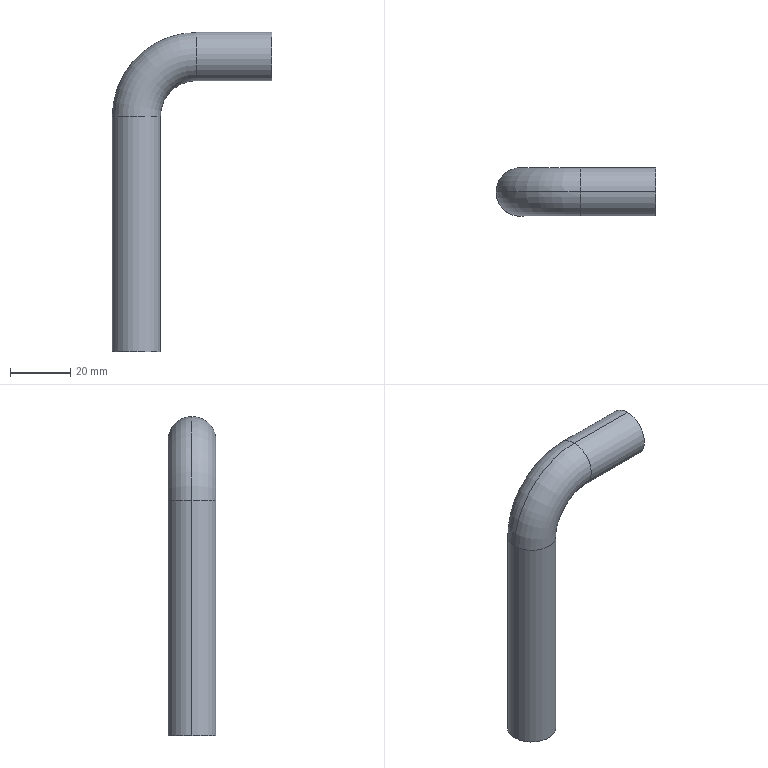Part | STEP file | copper tube 44 | 1 solid | 14 faces | box 53 x 16 x 106 mm | volume 7500 mm3 | cylinder 8 | torus 4 | plane 2 | commonest cylinder face diameters 13.6 x4 16 x4
STEP:
#1=CARTESIAN_POINT('',(0.,0.,0.));
#2=DIRECTION('',(0.,0.,1.));
#3=DIRECTION('',(1.,0.,0.));
#4=AXIS2_PLACEMENT_3D('',#1,#2,#3);
#5=CARTESIAN_POINT('',(6.8,0.,78.));
#6=VERTEX_POINT('',#5);
#7=CARTESIAN_POINT('',(20.,0.,91.2));
#8=VERTEX_POINT('',#7);
#9=CARTESIAN_POINT('',(20.,0.,78.));
#10=DIRECTION('',(0.,1.,0.));
#11=DIRECTION('',(0.,0.,1.));
#12=AXIS2_PLACEMENT_3D('',#9,#10,#11);
#13=CIRCLE('',#12,13.2);
#14=CARTESIAN_POINT('',(20.,0.,78.));
#15=DIRECTION('',(0.,1.,0.));
#16=DIRECTION('',(0.,0.,1.));
#17=AXIS2_PLACEMENT_3D('',#14,#15,#16);
#18=TOROIDAL_SURFACE('',#17,20.,6.8);
#19=CARTESIAN_POINT('',(0.,3.142));
#20=DIRECTION('',(1.,0.));
#21=VECTOR('',#20,1.);
#22=LINE('',#19,#21);
#23=(GEOMETRIC_REPRESENTATION_CONTEXT(2)PARAMETRIC_REPRESENTATION_CONTEXT()REPRESENTATION_CONTEXT('',''));
#24=DEFINITIONAL_REPRESENTATION('',(#22),#23);
#25=PCURVE('',#18,#24);
#26=CARTESIAN_POINT('',(20.,0.,78.));
#27=DIRECTION('',(0.,1.,0.));
#28=DIRECTION('',(0.,0.,1.));
#29=AXIS2_PLACEMENT_3D('',#26,#27,#28);
#30=TOROIDAL_SURFACE('',#29,20.,6.8);
#31=CARTESIAN_POINT('',(0.,3.142));
#32=DIRECTION('',(1.,0.));
#33=VECTOR('',#32,1.);
#34=LINE('',#31,#33);
#35=(GEOMETRIC_REPRESENTATION_CONTEXT(2)PARAMETRIC_REPRESENTATION_CONTEXT()REPRESENTATION_CONTEXT('',''));
#36=DEFINITIONAL_REPRESENTATION('',(#34),#35);
#37=PCURVE('',#30,#36);
#38=SURFACE_CURVE('',#13,(#25,#37),.PCURVE_S1.);
#39=EDGE_CURVE('',#6,#8,#38,.T.);
#40=ORIENTED_EDGE('',*,*,#39,.T.);
#41=CARTESIAN_POINT('',(20.,0.,104.8));
#42=VERTEX_POINT('',#41);
#43=CARTESIAN_POINT('',(20.,0.,98.));
#44=DIRECTION('',(1.,0.,0.));
#45=DIRECTION('',(0.,0.,-1.));
#46=AXIS2_PLACEMENT_3D('',#43,#44,#45);
#47=CIRCLE('',#46,6.8);
#48=CARTESIAN_POINT('',(6.283,9.425));
#49=DIRECTION('',(0.,-1.));
#50=VECTOR('',#49,1.);
#51=LINE('',#48,#50);
#52=(GEOMETRIC_REPRESENTATION_CONTEXT(2)PARAMETRIC_REPRESENTATION_CONTEXT()REPRESENTATION_CONTEXT('',''));
#53=DEFINITIONAL_REPRESENTATION('',(#51),#52);
#54=PCURVE('',#18,#53);
#55=CARTESIAN_POINT('',(20.,0.,98.));
#56=DIRECTION('',(1.,0.,0.));
#57=DIRECTION('',(0.,0.,-1.));
#58=AXIS2_PLACEMENT_3D('',#55,#56,#57);
#59=CYLINDRICAL_SURFACE('',#58,6.8);
#60=CARTESIAN_POINT('',(0.,0.));
#61=DIRECTION('',(1.,0.));
#62=VECTOR('',#61,1.);
#63=LINE('',#60,#62);
#64=(GEOMETRIC_REPRESENTATION_CONTEXT(2)PARAMETRIC_REPRESENTATION_CONTEXT()REPRESENTATION_CONTEXT('',''));
#65=DEFINITIONAL_REPRESENTATION('',(#63),#64);
#66=PCURVE('',#59,#65);
#67=SURFACE_CURVE('',#47,(#54,#66),.PCURVE_S1.);
#68=EDGE_CURVE('',#42,#8,#67,.T.);
#69=ORIENTED_EDGE('',*,*,#68,.F.);
#70=CARTESIAN_POINT('',(-6.8,0.,78.));
#71=VERTEX_POINT('',#70);
#72=CARTESIAN_POINT('',(20.,0.,78.));
#73=DIRECTION('',(0.,1.,0.));
#74=DIRECTION('',(0.,0.,1.));
#75=AXIS2_PLACEMENT_3D('',#72,#73,#74);
#76=CIRCLE('',#75,26.8);
#77=CARTESIAN_POINT('',(0.,6.283));
#78=DIRECTION('',(1.,0.));
#79=VECTOR('',#78,1.);
#80=LINE('',#77,#79);
#81=(GEOMETRIC_REPRESENTATION_CONTEXT(2)PARAMETRIC_REPRESENTATION_CONTEXT()REPRESENTATION_CONTEXT('',''));
#82=DEFINITIONAL_REPRESENTATION('',(#80),#81);
#83=PCURVE('',#18,#82);
#84=CARTESIAN_POINT('',(0.,0.));
#85=DIRECTION('',(1.,0.));
#86=VECTOR('',#85,1.);
#87=LINE('',#84,#86);
#88=(GEOMETRIC_REPRESENTATION_CONTEXT(2)PARAMETRIC_REPRESENTATION_CONTEXT()REPRESENTATION_CONTEXT('',''));
#89=DEFINITIONAL_REPRESENTATION('',(#87),#88);
#90=PCURVE('',#30,#89);
#91=SURFACE_CURVE('',#76,(#83,#90),.PCURVE_S1.);
#92=EDGE_CURVE('',#71,#42,#91,.T.);
#93=ORIENTED_EDGE('',*,*,#92,.F.);
#94=CARTESIAN_POINT('',(0.,0.,78.));
#95=DIRECTION('',(0.,0.,1.));
#96=DIRECTION('',(-1.,0.,0.));
#97=AXIS2_PLACEMENT_3D('',#94,#95,#96);
#98=CIRCLE('',#97,6.8);
#99=CARTESIAN_POINT('',(4.712,6.283));
#100=DIRECTION('',(0.,-1.));
#101=VECTOR('',#100,1.);
#102=LINE('',#99,#101);
#103=(GEOMETRIC_REPRESENTATION_CONTEXT(2)PARAMETRIC_REPRESENTATION_CONTEXT()REPRESENTATION_CONTEXT('',''));
#104=DEFINITIONAL_REPRESENTATION('',(#102),#103);
#105=PCURVE('',#18,#104);
#106=CARTESIAN_POINT('',(0.,0.,78.));
#107=DIRECTION('',(0.,0.,-1.));
#108=DIRECTION('',(-1.,0.,0.));
#109=AXIS2_PLACEMENT_3D('',#106,#107,#108);
#110=CYLINDRICAL_SURFACE('',#109,6.8);
#111=CARTESIAN_POINT('',(6.283,0.));
#112=DIRECTION('',(-1.,0.));
#113=VECTOR('',#112,1.);
#114=LINE('',#111,#113);
#115=(GEOMETRIC_REPRESENTATION_CONTEXT(2)PARAMETRIC_REPRESENTATION_CONTEXT()REPRESENTATION_CONTEXT('',''));
#116=DEFINITIONAL_REPRESENTATION('',(#114),#115);
#117=PCURVE('',#110,#116);
#118=SURFACE_CURVE('',#98,(#105,#117),.PCURVE_S1.);
#119=EDGE_CURVE('',#71,#6,#118,.T.);
#120=ORIENTED_EDGE('',*,*,#119,.T.);
#121=EDGE_LOOP('',(#40,#69,#93,#120));
#122=FACE_BOUND('',#121,.F.);
#123=ADVANCED_FACE('',(#122),#18,.F.);
#124=CARTESIAN_POINT('',(8.,0.,78.));
#125=VERTEX_POINT('',#124);
#126=CARTESIAN_POINT('',(-8.,0.,78.));
#127=VERTEX_POINT('',#126);
#128=CARTESIAN_POINT('',(0.,0.,78.));
#129=DIRECTION('',(0.,0.,1.));
#130=DIRECTION('',(1.,0.,0.));
#131=AXIS2_PLACEMENT_3D('',#128,#129,#130);
#132=CIRCLE('',#131,8.);
#133=CARTESIAN_POINT('',(20.,0.,78.));
#134=DIRECTION('',(0.,1.,0.));
#135=DIRECTION('',(0.,0.,1.));
#136=AXIS2_PLACEMENT_3D('',#133,#134,#135);
#137=TOROIDAL_SURFACE('',#136,20.,8.);
#138=CARTESIAN_POINT('',(4.712,3.142));
#139=DIRECTION('',(0.,-1.));
#140=VECTOR('',#139,1.);
#141=LINE('',#138,#140);
#142=(GEOMETRIC_REPRESENTATION_CONTEXT(2)PARAMETRIC_REPRESENTATION_CONTEXT()REPRESENTATION_CONTEXT('',''));
#143=DEFINITIONAL_REPRESENTATION('',(#141),#142);
#144=PCURVE('',#137,#143);
#145=CARTESIAN_POINT('',(0.,0.,78.));
#146=DIRECTION('',(0.,0.,-1.));
#147=DIRECTION('',(-1.,0.,0.));
#148=AXIS2_PLACEMENT_3D('',#145,#146,#147);
#149=CYLINDRICAL_SURFACE('',#148,8.);
#150=CARTESIAN_POINT('',(3.142,0.));
#151=DIRECTION('',(-1.,0.));
#152=VECTOR('',#151,1.);
#153=LINE('',#150,#152);
#154=(GEOMETRIC_REPRESENTATION_CONTEXT(2)PARAMETRIC_REPRESENTATION_CONTEXT()REPRESENTATION_CONTEXT('',''));
#155=DEFINITIONAL_REPRESENTATION('',(#153),#154);
#156=PCURVE('',#149,#155);
#157=SURFACE_CURVE('',#132,(#144,#156),.PCURVE_S1.);
#158=EDGE_CURVE('',#125,#127,#157,.T.);
#159=ORIENTED_EDGE('',*,*,#158,.T.);
#160=CARTESIAN_POINT('',(20.,0.,106.));
#161=VERTEX_POINT('',#160);
#162=CARTESIAN_POINT('',(20.,0.,78.));
#163=DIRECTION('',(0.,1.,0.));
#164=DIRECTION('',(0.,0.,1.));
#165=AXIS2_PLACEMENT_3D('',#162,#163,#164);
#166=CIRCLE('',#165,28.);
#167=CARTESIAN_POINT('',(0.,0.));
#168=DIRECTION('',(1.,0.));
#169=VECTOR('',#168,1.);
#170=LINE('',#167,#169);
#171=(GEOMETRIC_REPRESENTATION_CONTEXT(2)PARAMETRIC_REPRESENTATION_CONTEXT()REPRESENTATION_CONTEXT('',''));
#172=DEFINITIONAL_REPRESENTATION('',(#170),#171);
#173=PCURVE('',#137,#172);
#174=CARTESIAN_POINT('',(20.,0.,78.));
#175=DIRECTION('',(0.,1.,0.));
#176=DIRECTION('',(0.,0.,1.));
#177=AXIS2_PLACEMENT_3D('',#174,#175,#176);
#178=TOROIDAL_SURFACE('',#177,20.,8.);
#179=CARTESIAN_POINT('',(0.,6.283));
#180=DIRECTION('',(1.,0.));
#181=VECTOR('',#180,1.);
#182=LINE('',#179,#181);
#183=(GEOMETRIC_REPRESENTATION_CONTEXT(2)PARAMETRIC_REPRESENTATION_CONTEXT()REPRESENTATION_CONTEXT('',''));
#184=DEFINITIONAL_REPRESENTATION('',(#182),#183);
#185=PCURVE('',#178,#184);
#186=SURFACE_CURVE('',#166,(#173,#185),.PCURVE_S1.);
#187=EDGE_CURVE('',#127,#161,#186,.T.);
#188=ORIENTED_EDGE('',*,*,#187,.T.);
#189=CARTESIAN_POINT('',(20.,0.,90.));
#190=VERTEX_POINT('',#189);
#191=CARTESIAN_POINT('',(20.,0.,98.));
#192=DIRECTION('',(1.,0.,0.));
#193=DIRECTION('',(0.,0.,-1.));
#194=AXIS2_PLACEMENT_3D('',#191,#192,#193);
#195=CIRCLE('',#194,8.);
#196=CARTESIAN_POINT('',(6.283,3.142));
#197=DIRECTION('',(0.,-1.));
#198=VECTOR('',#197,1.);
#199=LINE('',#196,#198);
#200=(GEOMETRIC_REPRESENTATION_CONTEXT(2)PARAMETRIC_REPRESENTATION_CONTEXT()REPRESENTATION_CONTEXT('',''));
#201=DEFINITIONAL_REPRESENTATION('',(#199),#200);
#202=PCURVE('',#137,#201);
#203=CARTESIAN_POINT('',(20.,0.,98.));
#204=DIRECTION('',(1.,0.,0.));
#205=DIRECTION('',(0.,0.,-1.));
#206=AXIS2_PLACEMENT_3D('',#203,#204,#205);
#207=CYLINDRICAL_SURFACE('',#206,8.);
#208=CARTESIAN_POINT('',(0.,0.));
#209=DIRECTION('',(1.,0.));
#210=VECTOR('',#209,1.);
#211=LINE('',#208,#210);
#212=(GEOMETRIC_REPRESENTATION_CONTEXT(2)PARAMETRIC_REPRESENTATION_CONTEXT()REPRESENTATION_CONTEXT('',''));
#213=DEFINITIONAL_REPRESENTATION('',(#211),#212);
#214=PCURVE('',#207,#213);
#215=SURFACE_CURVE('',#195,(#202,#214),.PCURVE_S1.);
#216=EDGE_CURVE('',#190,#161,#215,.T.);
#217=ORIENTED_EDGE('',*,*,#216,.F.);
#218=CARTESIAN_POINT('',(20.,0.,78.));
#219=DIRECTION('',(0.,1.,0.));
#220=DIRECTION('',(0.,0.,1.));
#221=AXIS2_PLACEMENT_3D('',#218,#219,#220);
#222=CIRCLE('',#221,12.);
#223=CARTESIAN_POINT('',(0.,3.142));
#224=DIRECTION('',(1.,0.));
#225=VECTOR('',#224,1.);
#226=LINE('',#223,#225);
#227=(GEOMETRIC_REPRESENTATION_CONTEXT(2)PARAMETRIC_REPRESENTATION_CONTEXT()REPRESENTATION_CONTEXT('',''));
#228=DEFINITIONAL_REPRESENTATION('',(#226),#227);
#229=PCURVE('',#137,#228);
#230=CARTESIAN_POINT('',(0.,3.142));
#231=DIRECTION('',(1.,0.));
#232=VECTOR('',#231,1.);
#233=LINE('',#230,#232);
#234=(GEOMETRIC_REPRESENTATION_CONTEXT(2)PARAMETRIC_REPRESENTATION_CONTEXT()REPRESENTATION_CONTEXT('',''));
#235=DEFINITIONAL_REPRESENTATION('',(#233),#234);
#236=PCURVE('',#178,#235);
#237=SURFACE_CURVE('',#222,(#229,#236),.PCURVE_S1.);
#238=EDGE_CURVE('',#125,#190,#237,.T.);
#239=ORIENTED_EDGE('',*,*,#238,.F.);
#240=EDGE_LOOP('',(#159,#188,#217,#239));
#241=FACE_BOUND('',#240,.T.);
#242=ADVANCED_FACE('',(#241),#137,.T.);
#243=CARTESIAN_POINT('',(-6.8,0.,0.));
#244=VERTEX_POINT('',#243);
#245=CARTESIAN_POINT('',(-6.8,0.,78.));
#246=DIRECTION('',(0.,0.,-1.));
#247=VECTOR('',#246,1.);
#248=LINE('',#245,#247);
#249=CARTESIAN_POINT('',(6.283,0.));
#250=DIRECTION('',(0.,1.));
#251=VECTOR('',#250,1.);
#252=LINE('',#249,#251);
#253=(GEOMETRIC_REPRESENTATION_CONTEXT(2)PARAMETRIC_REPRESENTATION_CONTEXT()REPRESENTATION_CONTEXT('',''));
#254=DEFINITIONAL_REPRESENTATION('',(#252),#253);
#255=PCURVE('',#110,#254);
#256=CARTESIAN_POINT('',(0.,0.,78.));
#257=DIRECTION('',(0.,0.,-1.));
#258=DIRECTION('',(-1.,0.,0.));
#259=AXIS2_PLACEMENT_3D('',#256,#257,#258);
#260=CYLINDRICAL_SURFACE('',#259,6.8);
#261=CARTESIAN_POINT('',(0.,0.));
#262=DIRECTION('',(0.,1.));
#263=VECTOR('',#262,1.);
#264=LINE('',#261,#263);
#265=(GEOMETRIC_REPRESENTATION_CONTEXT(2)PARAMETRIC_REPRESENTATION_CONTEXT()REPRESENTATION_CONTEXT('',''));
#266=DEFINITIONAL_REPRESENTATION('',(#264),#265);
#267=PCURVE('',#260,#266);
#268=SURFACE_CURVE('',#248,(#255,#267),.PCURVE_S1.);
#269=EDGE_CURVE('',#71,#244,#268,.T.);
#270=ORIENTED_EDGE('',*,*,#269,.T.);
#271=CARTESIAN_POINT('',(6.8,0.,0.));
#272=VERTEX_POINT('',#271);
#273=CARTESIAN_POINT('',(0.,0.,0.));
#274=DIRECTION('',(0.,0.,1.));
#275=DIRECTION('',(1.,0.,0.));
#276=AXIS2_PLACEMENT_3D('',#273,#274,#275);
#277=CIRCLE('',#276,6.8);
#278=CARTESIAN_POINT('',(9.425,78.));
#279=DIRECTION('',(-1.,0.));
#280=VECTOR('',#279,1.);
#281=LINE('',#278,#280);
#282=(GEOMETRIC_REPRESENTATION_CONTEXT(2)PARAMETRIC_REPRESENTATION_CONTEXT()REPRESENTATION_CONTEXT('',''));
#283=DEFINITIONAL_REPRESENTATION('',(#281),#282);
#284=PCURVE('',#110,#283);
#285=CARTESIAN_POINT('',(0.,0.,0.));
#286=DIRECTION('',(0.,0.,1.));
#287=DIRECTION('',(1.,0.,0.));
#288=AXIS2_PLACEMENT_3D('',#285,#286,#287);
#289=PLANE('',#288);
#290=CARTESIAN_POINT('',(0.,0.));
#291=DIRECTION('',(1.,0.));
#292=AXIS2_PLACEMENT_2D('',#290,#291);
#293=CIRCLE('',#292,6.8);
#294=(GEOMETRIC_REPRESENTATION_CONTEXT(2)PARAMETRIC_REPRESENTATION_CONTEXT()REPRESENTATION_CONTEXT('',''));
#295=DEFINITIONAL_REPRESENTATION('',(#293),#294);
#296=PCURVE('',#289,#295);
#297=SURFACE_CURVE('',#277,(#284,#296),.PCURVE_S1.);
#298=EDGE_CURVE('',#244,#272,#297,.T.);
#299=ORIENTED_EDGE('',*,*,#298,.T.);
#300=CARTESIAN_POINT('',(6.8,0.,78.));
#301=DIRECTION('',(0.,0.,-1.));
#302=VECTOR('',#301,1.);
#303=LINE('',#300,#302);
#304=CARTESIAN_POINT('',(3.142,0.));
#305=DIRECTION('',(0.,1.));
#306=VECTOR('',#305,1.);
#307=LINE('',#304,#306);
#308=(GEOMETRIC_REPRESENTATION_CONTEXT(2)PARAMETRIC_REPRESENTATION_CONTEXT()REPRESENTATION_CONTEXT('',''));
#309=DEFINITIONAL_REPRESENTATION('',(#307),#308);
#310=PCURVE('',#110,#309);
#311=CARTESIAN_POINT('',(3.142,0.));
#312=DIRECTION('',(0.,1.));
#313=VECTOR('',#312,1.);
#314=LINE('',#311,#313);
#315=(GEOMETRIC_REPRESENTATION_CONTEXT(2)PARAMETRIC_REPRESENTATION_CONTEXT()REPRESENTATION_CONTEXT('',''));
#316=DEFINITIONAL_REPRESENTATION('',(#314),#315);
#317=PCURVE('',#260,#316);
#318=SURFACE_CURVE('',#303,(#310,#317),.PCURVE_S1.);
#319=EDGE_CURVE('',#6,#272,#318,.T.);
#320=ORIENTED_EDGE('',*,*,#319,.F.);
#321=ORIENTED_EDGE('',*,*,#119,.F.);
#322=EDGE_LOOP('',(#270,#299,#320,#321));
#323=FACE_BOUND('',#322,.F.);
#324=ADVANCED_FACE('',(#323),#110,.F.);
#325=CARTESIAN_POINT('',(45.,0.,91.2));
#326=VERTEX_POINT('',#325);
#327=CARTESIAN_POINT('',(20.,0.,91.2));
#328=DIRECTION('',(1.,0.,0.));
#329=VECTOR('',#328,1.);
#330=LINE('',#327,#329);
#331=CARTESIAN_POINT('',(6.283,0.));
#332=DIRECTION('',(0.,1.));
#333=VECTOR('',#332,1.);
#334=LINE('',#331,#333);
#335=(GEOMETRIC_REPRESENTATION_CONTEXT(2)PARAMETRIC_REPRESENTATION_CONTEXT()REPRESENTATION_CONTEXT('',''));
#336=DEFINITIONAL_REPRESENTATION('',(#334),#335);
#337=PCURVE('',#59,#336);
#338=CARTESIAN_POINT('',(20.,0.,98.));
#339=DIRECTION('',(1.,0.,0.));
#340=DIRECTION('',(0.,0.,-1.));
#341=AXIS2_PLACEMENT_3D('',#338,#339,#340);
#342=CYLINDRICAL_SURFACE('',#341,6.8);
#343=CARTESIAN_POINT('',(0.,0.));
#344=DIRECTION('',(0.,1.));
#345=VECTOR('',#344,1.);
#346=LINE('',#343,#345);
#347=(GEOMETRIC_REPRESENTATION_CONTEXT(2)PARAMETRIC_REPRESENTATION_CONTEXT()REPRESENTATION_CONTEXT('',''));
#348=DEFINITIONAL_REPRESENTATION('',(#346),#347);
#349=PCURVE('',#342,#348);
#350=SURFACE_CURVE('',#330,(#337,#349),.PCURVE_S1.);
#351=EDGE_CURVE('',#8,#326,#350,.T.);
#352=ORIENTED_EDGE('',*,*,#351,.T.);
#353=CARTESIAN_POINT('',(45.,0.,104.8));
#354=VERTEX_POINT('',#353);
#355=CARTESIAN_POINT('',(45.,0.,98.));
#356=DIRECTION('',(1.,0.,0.));
#357=DIRECTION('',(0.,0.,-1.));
#358=AXIS2_PLACEMENT_3D('',#355,#356,#357);
#359=CIRCLE('',#358,6.8);
#360=CARTESIAN_POINT('',(0.,25.));
#361=DIRECTION('',(1.,0.));
#362=VECTOR('',#361,1.);
#363=LINE('',#360,#362);
#364=(GEOMETRIC_REPRESENTATION_CONTEXT(2)PARAMETRIC_REPRESENTATION_CONTEXT()REPRESENTATION_CONTEXT('',''));
#365=DEFINITIONAL_REPRESENTATION('',(#363),#364);
#366=PCURVE('',#59,#365);
#367=CARTESIAN_POINT('',(45.,0.,98.));
#368=DIRECTION('',(1.,0.,0.));
#369=DIRECTION('',(0.,0.,-1.));
#370=AXIS2_PLACEMENT_3D('',#367,#368,#369);
#371=PLANE('',#370);
#372=CARTESIAN_POINT('',(0.,0.));
#373=DIRECTION('',(1.,0.));
#374=AXIS2_PLACEMENT_2D('',#372,#373);
#375=CIRCLE('',#374,6.8);
#376=(GEOMETRIC_REPRESENTATION_CONTEXT(2)PARAMETRIC_REPRESENTATION_CONTEXT()REPRESENTATION_CONTEXT('',''));
#377=DEFINITIONAL_REPRESENTATION('',(#375),#376);
#378=PCURVE('',#371,#377);
#379=SURFACE_CURVE('',#359,(#366,#378),.PCURVE_S1.);
#380=EDGE_CURVE('',#354,#326,#379,.T.);
#381=ORIENTED_EDGE('',*,*,#380,.F.);
#382=CARTESIAN_POINT('',(20.,0.,104.8));
#383=DIRECTION('',(1.,0.,0.));
#384=VECTOR('',#383,1.);
#385=LINE('',#382,#384);
#386=CARTESIAN_POINT('',(3.142,0.));
#387=DIRECTION('',(0.,1.));
#388=VECTOR('',#387,1.);
#389=LINE('',#386,#388);
#390=(GEOMETRIC_REPRESENTATION_CONTEXT(2)PARAMETRIC_REPRESENTATION_CONTEXT()REPRESENTATION_CONTEXT('',''));
#391=DEFINITIONAL_REPRESENTATION('',(#389),#390);
#392=PCURVE('',#59,#391);
#393=CARTESIAN_POINT('',(3.142,0.));
#394=DIRECTION('',(0.,1.));
#395=VECTOR('',#394,1.);
#396=LINE('',#393,#395);
#397=(GEOMETRIC_REPRESENTATION_CONTEXT(2)PARAMETRIC_REPRESENTATION_CONTEXT()REPRESENTATION_CONTEXT('',''));
#398=DEFINITIONAL_REPRESENTATION('',(#396),#397);
#399=PCURVE('',#342,#398);
#400=SURFACE_CURVE('',#385,(#392,#399),.PCURVE_S1.);
#401=EDGE_CURVE('',#42,#354,#400,.T.);
#402=ORIENTED_EDGE('',*,*,#401,.F.);
#403=ORIENTED_EDGE('',*,*,#68,.T.);
#404=EDGE_LOOP('',(#352,#381,#402,#403));
#405=FACE_BOUND('',#404,.F.);
#406=ADVANCED_FACE('',(#405),#59,.F.);
#407=ORIENTED_EDGE('',*,*,#158,.F.);
#408=CARTESIAN_POINT('',(8.,0.,0.));
#409=VERTEX_POINT('',#408);
#410=CARTESIAN_POINT('',(8.,0.,78.));
#411=DIRECTION('',(0.,0.,-1.));
#412=VECTOR('',#411,1.);
#413=LINE('',#410,#412);
#414=CARTESIAN_POINT('',(3.142,0.));
#415=DIRECTION('',(0.,1.));
#416=VECTOR('',#415,1.);
#417=LINE('',#414,#416);
#418=(GEOMETRIC_REPRESENTATION_CONTEXT(2)PARAMETRIC_REPRESENTATION_CONTEXT()REPRESENTATION_CONTEXT('',''));
#419=DEFINITIONAL_REPRESENTATION('',(#417),#418);
#420=PCURVE('',#149,#419);
#421=CARTESIAN_POINT('',(0.,0.,78.));
#422=DIRECTION('',(0.,0.,-1.));
#423=DIRECTION('',(-1.,0.,0.));
#424=AXIS2_PLACEMENT_3D('',#421,#422,#423);
#425=CYLINDRICAL_SURFACE('',#424,8.);
#426=CARTESIAN_POINT('',(3.142,0.));
#427=DIRECTION('',(0.,1.));
#428=VECTOR('',#427,1.);
#429=LINE('',#426,#428);
#430=(GEOMETRIC_REPRESENTATION_CONTEXT(2)PARAMETRIC_REPRESENTATION_CONTEXT()REPRESENTATION_CONTEXT('',''));
#431=DEFINITIONAL_REPRESENTATION('',(#429),#430);
#432=PCURVE('',#425,#431);
#433=SURFACE_CURVE('',#413,(#420,#432),.PCURVE_S1.);
#434=EDGE_CURVE('',#125,#409,#433,.T.);
#435=ORIENTED_EDGE('',*,*,#434,.T.);
#436=CARTESIAN_POINT('',(-8.,0.,0.));
#437=VERTEX_POINT('',#436);
#438=CARTESIAN_POINT('',(0.,0.,0.));
#439=DIRECTION('',(0.,0.,1.));
#440=DIRECTION('',(1.,0.,0.));
#441=AXIS2_PLACEMENT_3D('',#438,#439,#440);
#442=CIRCLE('',#441,8.);
#443=CARTESIAN_POINT('',(3.142,78.));
#444=DIRECTION('',(-1.,0.));
#445=VECTOR('',#444,1.);
#446=LINE('',#443,#445);
#447=(GEOMETRIC_REPRESENTATION_CONTEXT(2)PARAMETRIC_REPRESENTATION_CONTEXT()REPRESENTATION_CONTEXT('',''));
#448=DEFINITIONAL_REPRESENTATION('',(#446),#447);
#449=PCURVE('',#149,#448);
#450=CARTESIAN_POINT('',(0.,0.));
#451=DIRECTION('',(1.,0.));
#452=AXIS2_PLACEMENT_2D('',#450,#451);
#453=CIRCLE('',#452,8.);
#454=(GEOMETRIC_REPRESENTATION_CONTEXT(2)PARAMETRIC_REPRESENTATION_CONTEXT()REPRESENTATION_CONTEXT('',''));
#455=DEFINITIONAL_REPRESENTATION('',(#453),#454);
#456=PCURVE('',#289,#455);
#457=SURFACE_CURVE('',#442,(#449,#456),.PCURVE_S1.);
#458=EDGE_CURVE('',#409,#437,#457,.T.);
#459=ORIENTED_EDGE('',*,*,#458,.T.);
#460=CARTESIAN_POINT('',(-8.,0.,78.));
#461=DIRECTION('',(0.,0.,-1.));
#462=VECTOR('',#461,1.);
#463=LINE('',#460,#462);
#464=CARTESIAN_POINT('',(0.,0.));
#465=DIRECTION('',(0.,1.));
#466=VECTOR('',#465,1.);
#467=LINE('',#464,#466);
#468=(GEOMETRIC_REPRESENTATION_CONTEXT(2)PARAMETRIC_REPRESENTATION_CONTEXT()REPRESENTATION_CONTEXT('',''));
#469=DEFINITIONAL_REPRESENTATION('',(#467),#468);
#470=PCURVE('',#149,#469);
#471=CARTESIAN_POINT('',(6.283,0.));
#472=DIRECTION('',(0.,1.));
#473=VECTOR('',#472,1.);
#474=LINE('',#471,#473);
#475=(GEOMETRIC_REPRESENTATION_CONTEXT(2)PARAMETRIC_REPRESENTATION_CONTEXT()REPRESENTATION_CONTEXT('',''));
#476=DEFINITIONAL_REPRESENTATION('',(#474),#475);
#477=PCURVE('',#425,#476);
#478=SURFACE_CURVE('',#463,(#470,#477),.PCURVE_S1.);
#479=EDGE_CURVE('',#127,#437,#478,.T.);
#480=ORIENTED_EDGE('',*,*,#479,.F.);
#481=EDGE_LOOP('',(#407,#435,#459,#480));
#482=FACE_BOUND('',#481,.T.);
#483=ADVANCED_FACE('',(#482),#149,.T.);
#484=ORIENTED_EDGE('',*,*,#216,.T.);
#485=CARTESIAN_POINT('',(45.,0.,106.));
#486=VERTEX_POINT('',#485);
#487=CARTESIAN_POINT('',(20.,0.,106.));
#488=DIRECTION('',(1.,0.,0.));
#489=VECTOR('',#488,1.);
#490=LINE('',#487,#489);
#491=CARTESIAN_POINT('',(3.142,0.));
#492=DIRECTION('',(0.,1.));
#493=VECTOR('',#492,1.);
#494=LINE('',#491,#493);
#495=(GEOMETRIC_REPRESENTATION_CONTEXT(2)PARAMETRIC_REPRESENTATION_CONTEXT()REPRESENTATION_CONTEXT('',''));
#496=DEFINITIONAL_REPRESENTATION('',(#494),#495);
#497=PCURVE('',#207,#496);
#498=CARTESIAN_POINT('',(20.,0.,98.));
#499=DIRECTION('',(1.,0.,0.));
#500=DIRECTION('',(0.,0.,-1.));
#501=AXIS2_PLACEMENT_3D('',#498,#499,#500);
#502=CYLINDRICAL_SURFACE('',#501,8.);
#503=CARTESIAN_POINT('',(3.142,0.));
#504=DIRECTION('',(0.,1.));
#505=VECTOR('',#504,1.);
#506=LINE('',#503,#505);
#507=(GEOMETRIC_REPRESENTATION_CONTEXT(2)PARAMETRIC_REPRESENTATION_CONTEXT()REPRESENTATION_CONTEXT('',''));
#508=DEFINITIONAL_REPRESENTATION('',(#506),#507);
#509=PCURVE('',#502,#508);
#510=SURFACE_CURVE('',#490,(#497,#509),.PCURVE_S1.);
#511=EDGE_CURVE('',#161,#486,#510,.T.);
#512=ORIENTED_EDGE('',*,*,#511,.T.);
#513=CARTESIAN_POINT('',(45.,0.,90.));
#514=VERTEX_POINT('',#513);
#515=CARTESIAN_POINT('',(45.,0.,98.));
#516=DIRECTION('',(1.,0.,0.));
#517=DIRECTION('',(0.,0.,-1.));
#518=AXIS2_PLACEMENT_3D('',#515,#516,#517);
#519=CIRCLE('',#518,8.);
#520=CARTESIAN_POINT('',(0.,25.));
#521=DIRECTION('',(1.,0.));
#522=VECTOR('',#521,1.);
#523=LINE('',#520,#522);
#524=(GEOMETRIC_REPRESENTATION_CONTEXT(2)PARAMETRIC_REPRESENTATION_CONTEXT()REPRESENTATION_CONTEXT('',''));
#525=DEFINITIONAL_REPRESENTATION('',(#523),#524);
#526=PCURVE('',#207,#525);
#527=CARTESIAN_POINT('',(0.,0.));
#528=DIRECTION('',(1.,0.));
#529=AXIS2_PLACEMENT_2D('',#527,#528);
#530=CIRCLE('',#529,8.);
#531=(GEOMETRIC_REPRESENTATION_CONTEXT(2)PARAMETRIC_REPRESENTATION_CONTEXT()REPRESENTATION_CONTEXT('',''));
#532=DEFINITIONAL_REPRESENTATION('',(#530),#531);
#533=PCURVE('',#371,#532);
#534=SURFACE_CURVE('',#519,(#526,#533),.PCURVE_S1.);
#535=EDGE_CURVE('',#514,#486,#534,.T.);
#536=ORIENTED_EDGE('',*,*,#535,.F.);
#537=CARTESIAN_POINT('',(20.,0.,90.));
#538=DIRECTION('',(1.,0.,0.));
#539=VECTOR('',#538,1.);
#540=LINE('',#537,#539);
#541=CARTESIAN_POINT('',(0.,0.));
#542=DIRECTION('',(0.,1.));
#543=VECTOR('',#542,1.);
#544=LINE('',#541,#543);
#545=(GEOMETRIC_REPRESENTATION_CONTEXT(2)PARAMETRIC_REPRESENTATION_CONTEXT()REPRESENTATION_CONTEXT('',''));
#546=DEFINITIONAL_REPRESENTATION('',(#544),#545);
#547=PCURVE('',#207,#546);
#548=CARTESIAN_POINT('',(6.283,0.));
#549=DIRECTION('',(0.,1.));
#550=VECTOR('',#549,1.);
#551=LINE('',#548,#550);
#552=(GEOMETRIC_REPRESENTATION_CONTEXT(2)PARAMETRIC_REPRESENTATION_CONTEXT()REPRESENTATION_CONTEXT('',''));
#553=DEFINITIONAL_REPRESENTATION('',(#551),#552);
#554=PCURVE('',#502,#553);
#555=SURFACE_CURVE('',#540,(#547,#554),.PCURVE_S1.);
#556=EDGE_CURVE('',#190,#514,#555,.T.);
#557=ORIENTED_EDGE('',*,*,#556,.F.);
#558=EDGE_LOOP('',(#484,#512,#536,#557));
#559=FACE_BOUND('',#558,.T.);
#560=ADVANCED_FACE('',(#559),#207,.T.);
#561=ORIENTED_EDGE('',*,*,#511,.F.);
#562=CARTESIAN_POINT('',(20.,0.,98.));
#563=DIRECTION('',(1.,0.,0.));
#564=DIRECTION('',(0.,0.,-1.));
#565=AXIS2_PLACEMENT_3D('',#562,#563,#564);
#566=CIRCLE('',#565,8.);
#567=CARTESIAN_POINT('',(0.,0.));
#568=DIRECTION('',(1.,0.));
#569=VECTOR('',#568,1.);
#570=LINE('',#567,#569);
#571=(GEOMETRIC_REPRESENTATION_CONTEXT(2)PARAMETRIC_REPRESENTATION_CONTEXT()REPRESENTATION_CONTEXT('',''));
#572=DEFINITIONAL_REPRESENTATION('',(#570),#571);
#573=PCURVE('',#502,#572);
#574=CARTESIAN_POINT('',(6.283,9.425));
#575=DIRECTION('',(0.,-1.));
#576=VECTOR('',#575,1.);
#577=LINE('',#574,#576);
#578=(GEOMETRIC_REPRESENTATION_CONTEXT(2)PARAMETRIC_REPRESENTATION_CONTEXT()REPRESENTATION_CONTEXT('',''));
#579=DEFINITIONAL_REPRESENTATION('',(#577),#578);
#580=PCURVE('',#178,#579);
#581=SURFACE_CURVE('',#566,(#573,#580),.PCURVE_S1.);
#582=EDGE_CURVE('',#161,#190,#581,.T.);
#583=ORIENTED_EDGE('',*,*,#582,.T.);
#584=ORIENTED_EDGE('',*,*,#556,.T.);
#585=CARTESIAN_POINT('',(45.,0.,98.));
#586=DIRECTION('',(1.,0.,0.));
#587=DIRECTION('',(0.,0.,-1.));
#588=AXIS2_PLACEMENT_3D('',#585,#586,#587);
#589=CIRCLE('',#588,8.);
#590=CARTESIAN_POINT('',(0.,25.));
#591=DIRECTION('',(1.,0.));
#592=VECTOR('',#591,1.);
#593=LINE('',#590,#592);
#594=(GEOMETRIC_REPRESENTATION_CONTEXT(2)PARAMETRIC_REPRESENTATION_CONTEXT()REPRESENTATION_CONTEXT('',''));
#595=DEFINITIONAL_REPRESENTATION('',(#593),#594);
#596=PCURVE('',#502,#595);
#597=CARTESIAN_POINT('',(0.,0.));
#598=DIRECTION('',(1.,0.));
#599=AXIS2_PLACEMENT_2D('',#597,#598);
#600=CIRCLE('',#599,8.);
#601=(GEOMETRIC_REPRESENTATION_CONTEXT(2)PARAMETRIC_REPRESENTATION_CONTEXT()REPRESENTATION_CONTEXT('',''));
#602=DEFINITIONAL_REPRESENTATION('',(#600),#601);
#603=PCURVE('',#371,#602);
#604=SURFACE_CURVE('',#589,(#596,#603),.PCURVE_S1.);
#605=EDGE_CURVE('',#486,#514,#604,.T.);
#606=ORIENTED_EDGE('',*,*,#605,.F.);
#607=EDGE_LOOP('',(#561,#583,#584,#606));
#608=FACE_BOUND('',#607,.T.);
#609=ADVANCED_FACE('',(#608),#502,.T.);
#610=ORIENTED_EDGE('',*,*,#187,.F.);
#611=CARTESIAN_POINT('',(0.,0.,78.));
#612=DIRECTION('',(0.,0.,1.));
#613=DIRECTION('',(1.,0.,0.));
#614=AXIS2_PLACEMENT_3D('',#611,#612,#613);
#615=CIRCLE('',#614,8.);
#616=CARTESIAN_POINT('',(4.712,9.425));
#617=DIRECTION('',(0.,-1.));
#618=VECTOR('',#617,1.);
#619=LINE('',#616,#618);
#620=(GEOMETRIC_REPRESENTATION_CONTEXT(2)PARAMETRIC_REPRESENTATION_CONTEXT()REPRESENTATION_CONTEXT('',''));
#621=DEFINITIONAL_REPRESENTATION('',(#619),#620);
#622=PCURVE('',#178,#621);
#623=CARTESIAN_POINT('',(9.425,0.));
#624=DIRECTION('',(-1.,0.));
#625=VECTOR('',#624,1.);
#626=LINE('',#623,#625);
#627=(GEOMETRIC_REPRESENTATION_CONTEXT(2)PARAMETRIC_REPRESENTATION_CONTEXT()REPRESENTATION_CONTEXT('',''));
#628=DEFINITIONAL_REPRESENTATION('',(#626),#627);
#629=PCURVE('',#425,#628);
#630=SURFACE_CURVE('',#615,(#622,#629),.PCURVE_S1.);
#631=EDGE_CURVE('',#127,#125,#630,.T.);
#632=ORIENTED_EDGE('',*,*,#631,.T.);
#633=ORIENTED_EDGE('',*,*,#238,.T.);
#634=ORIENTED_EDGE('',*,*,#582,.F.);
#635=EDGE_LOOP('',(#610,#632,#633,#634));
#636=FACE_BOUND('',#635,.T.);
#637=ADVANCED_FACE('',(#636),#178,.T.);
#638=ORIENTED_EDGE('',*,*,#434,.F.);
#639=ORIENTED_EDGE('',*,*,#631,.F.);
#640=ORIENTED_EDGE('',*,*,#479,.T.);
#641=CARTESIAN_POINT('',(0.,0.,0.));
#642=DIRECTION('',(0.,0.,1.));
#643=DIRECTION('',(1.,0.,0.));
#644=AXIS2_PLACEMENT_3D('',#641,#642,#643);
#645=CIRCLE('',#644,8.);
#646=CARTESIAN_POINT('',(9.425,78.));
#647=DIRECTION('',(-1.,0.));
#648=VECTOR('',#647,1.);
#649=LINE('',#646,#648);
#650=(GEOMETRIC_REPRESENTATION_CONTEXT(2)PARAMETRIC_REPRESENTATION_CONTEXT()REPRESENTATION_CONTEXT('',''));
#651=DEFINITIONAL_REPRESENTATION('',(#649),#650);
#652=PCURVE('',#425,#651);
#653=CARTESIAN_POINT('',(0.,0.));
#654=DIRECTION('',(1.,0.));
#655=AXIS2_PLACEMENT_2D('',#653,#654);
#656=CIRCLE('',#655,8.);
#657=(GEOMETRIC_REPRESENTATION_CONTEXT(2)PARAMETRIC_REPRESENTATION_CONTEXT()REPRESENTATION_CONTEXT('',''));
#658=DEFINITIONAL_REPRESENTATION('',(#656),#657);
#659=PCURVE('',#289,#658);
#660=SURFACE_CURVE('',#645,(#652,#659),.PCURVE_S1.);
#661=EDGE_CURVE('',#437,#409,#660,.T.);
#662=ORIENTED_EDGE('',*,*,#661,.T.);
#663=EDGE_LOOP('',(#638,#639,#640,#662));
#664=FACE_BOUND('',#663,.T.);
#665=ADVANCED_FACE('',(#664),#425,.T.);
#666=CARTESIAN_POINT('',(45.,0.,98.));
#667=DIRECTION('',(1.,0.,0.));
#668=DIRECTION('',(0.,0.,-1.));
#669=AXIS2_PLACEMENT_3D('',#666,#667,#668);
#670=CIRCLE('',#669,6.8);
#671=CARTESIAN_POINT('',(0.,0.));
#672=DIRECTION('',(1.,0.));
#673=AXIS2_PLACEMENT_2D('',#671,#672);
#674=CIRCLE('',#673,6.8);
#675=(GEOMETRIC_REPRESENTATION_CONTEXT(2)PARAMETRIC_REPRESENTATION_CONTEXT()REPRESENTATION_CONTEXT('',''));
#676=DEFINITIONAL_REPRESENTATION('',(#674),#675);
#677=PCURVE('',#371,#676);
#678=CARTESIAN_POINT('',(0.,25.));
#679=DIRECTION('',(1.,0.));
#680=VECTOR('',#679,1.);
#681=LINE('',#678,#680);
#682=(GEOMETRIC_REPRESENTATION_CONTEXT(2)PARAMETRIC_REPRESENTATION_CONTEXT()REPRESENTATION_CONTEXT('',''));
#683=DEFINITIONAL_REPRESENTATION('',(#681),#682);
#684=PCURVE('',#342,#683);
#685=SURFACE_CURVE('',#670,(#677,#684),.PCURVE_S1.);
#686=EDGE_CURVE('',#326,#354,#685,.T.);
#687=ORIENTED_EDGE('',*,*,#686,.F.);
#688=ORIENTED_EDGE('',*,*,#380,.F.);
#689=EDGE_LOOP('',(#687,#688));
#690=FACE_BOUND('',#689,.T.);
#691=ORIENTED_EDGE('',*,*,#535,.T.);
#692=ORIENTED_EDGE('',*,*,#605,.T.);
#693=EDGE_LOOP('',(#691,#692));
#694=FACE_BOUND('',#693,.T.);
#695=ADVANCED_FACE('',(#690,#694),#371,.T.);
#696=ORIENTED_EDGE('',*,*,#298,.T.);
#697=CARTESIAN_POINT('',(0.,0.,0.));
#698=DIRECTION('',(0.,0.,1.));
#699=DIRECTION('',(1.,0.,0.));
#700=AXIS2_PLACEMENT_3D('',#697,#698,#699);
#701=CIRCLE('',#700,6.8);
#702=CARTESIAN_POINT('',(0.,0.));
#703=DIRECTION('',(1.,0.));
#704=AXIS2_PLACEMENT_2D('',#702,#703);
#705=CIRCLE('',#704,6.8);
#706=(GEOMETRIC_REPRESENTATION_CONTEXT(2)PARAMETRIC_REPRESENTATION_CONTEXT()REPRESENTATION_CONTEXT('',''));
#707=DEFINITIONAL_REPRESENTATION('',(#705),#706);
#708=PCURVE('',#289,#707);
#709=CARTESIAN_POINT('',(3.142,78.));
#710=DIRECTION('',(-1.,0.));
#711=VECTOR('',#710,1.);
#712=LINE('',#709,#711);
#713=(GEOMETRIC_REPRESENTATION_CONTEXT(2)PARAMETRIC_REPRESENTATION_CONTEXT()REPRESENTATION_CONTEXT('',''));
#714=DEFINITIONAL_REPRESENTATION('',(#712),#713);
#715=PCURVE('',#260,#714);
#716=SURFACE_CURVE('',#701,(#708,#715),.PCURVE_S1.);
#717=EDGE_CURVE('',#272,#244,#716,.T.);
#718=ORIENTED_EDGE('',*,*,#717,.T.);
#719=EDGE_LOOP('',(#696,#718));
#720=FACE_BOUND('',#719,.T.);
#721=ORIENTED_EDGE('',*,*,#661,.F.);
#722=ORIENTED_EDGE('',*,*,#458,.F.);
#723=EDGE_LOOP('',(#721,#722));
#724=FACE_BOUND('',#723,.T.);
#725=ADVANCED_FACE('',(#720,#724),#289,.F.);
#726=ORIENTED_EDGE('',*,*,#686,.F.);
#727=ORIENTED_EDGE('',*,*,#351,.F.);
#728=CARTESIAN_POINT('',(20.,0.,98.));
#729=DIRECTION('',(1.,0.,0.));
#730=DIRECTION('',(0.,0.,-1.));
#731=AXIS2_PLACEMENT_3D('',#728,#729,#730);
#732=CIRCLE('',#731,6.8);
#733=CARTESIAN_POINT('',(0.,0.));
#734=DIRECTION('',(1.,0.));
#735=VECTOR('',#734,1.);
#736=LINE('',#733,#735);
#737=(GEOMETRIC_REPRESENTATION_CONTEXT(2)PARAMETRIC_REPRESENTATION_CONTEXT()REPRESENTATION_CONTEXT('',''));
#738=DEFINITIONAL_REPRESENTATION('',(#736),#737);
#739=PCURVE('',#342,#738);
#740=CARTESIAN_POINT('',(6.283,3.142));
#741=DIRECTION('',(0.,-1.));
#742=VECTOR('',#741,1.);
#743=LINE('',#740,#742);
#744=(GEOMETRIC_REPRESENTATION_CONTEXT(2)PARAMETRIC_REPRESENTATION_CONTEXT()REPRESENTATION_CONTEXT('',''));
#745=DEFINITIONAL_REPRESENTATION('',(#743),#744);
#746=PCURVE('',#30,#745);
#747=SURFACE_CURVE('',#732,(#739,#746),.PCURVE_S1.);
#748=EDGE_CURVE('',#8,#42,#747,.T.);
#749=ORIENTED_EDGE('',*,*,#748,.T.);
#750=ORIENTED_EDGE('',*,*,#401,.T.);
#751=EDGE_LOOP('',(#726,#727,#749,#750));
#752=FACE_BOUND('',#751,.F.);
#753=ADVANCED_FACE('',(#752),#342,.F.);
#754=ORIENTED_EDGE('',*,*,#748,.F.);
#755=ORIENTED_EDGE('',*,*,#39,.F.);
#756=CARTESIAN_POINT('',(0.,0.,78.));
#757=DIRECTION('',(0.,0.,1.));
#758=DIRECTION('',(-1.,0.,0.));
#759=AXIS2_PLACEMENT_3D('',#756,#757,#758);
#760=CIRCLE('',#759,6.8);
#761=CARTESIAN_POINT('',(4.712,6.283));
#762=DIRECTION('',(0.,-1.));
#763=VECTOR('',#762,1.);
#764=LINE('',#761,#763);
#765=(GEOMETRIC_REPRESENTATION_CONTEXT(2)PARAMETRIC_REPRESENTATION_CONTEXT()REPRESENTATION_CONTEXT('',''));
#766=DEFINITIONAL_REPRESENTATION('',(#764),#765);
#767=PCURVE('',#30,#766);
#768=CARTESIAN_POINT('',(6.283,0.));
#769=DIRECTION('',(-1.,0.));
#770=VECTOR('',#769,1.);
#771=LINE('',#768,#770);
#772=(GEOMETRIC_REPRESENTATION_CONTEXT(2)PARAMETRIC_REPRESENTATION_CONTEXT()REPRESENTATION_CONTEXT('',''));
#773=DEFINITIONAL_REPRESENTATION('',(#771),#772);
#774=PCURVE('',#260,#773);
#775=SURFACE_CURVE('',#760,(#767,#774),.PCURVE_S1.);
#776=EDGE_CURVE('',#6,#71,#775,.T.);
#777=ORIENTED_EDGE('',*,*,#776,.T.);
#778=ORIENTED_EDGE('',*,*,#92,.T.);
#779=EDGE_LOOP('',(#754,#755,#777,#778));
#780=FACE_BOUND('',#779,.F.);
#781=ADVANCED_FACE('',(#780),#30,.F.);
#782=ORIENTED_EDGE('',*,*,#717,.T.);
#783=ORIENTED_EDGE('',*,*,#269,.F.);
#784=ORIENTED_EDGE('',*,*,#776,.F.);
#785=ORIENTED_EDGE('',*,*,#319,.T.);
#786=EDGE_LOOP('',(#782,#783,#784,#785));
#787=FACE_BOUND('',#786,.F.);
#788=ADVANCED_FACE('',(#787),#260,.F.);
#789=CLOSED_SHELL('',(#123,#242,#324,#406,#483,#560,#609,#637,#665,#695,#725,#753,#781,#788));
#790=MANIFOLD_SOLID_BREP('',#789);
#791=(LENGTH_UNIT()NAMED_UNIT(*)SI_UNIT(.MILLI.,.METRE.));
#792=UNCERTAINTY_MEASURE_WITH_UNIT(LENGTH_MEASURE(0.0000001),#791,'','');
#793=(NAMED_UNIT(*)PLANE_ANGLE_UNIT()SI_UNIT($,.RADIAN.));
#794=(NAMED_UNIT(*)SI_UNIT($,.STERADIAN.)SOLID_ANGLE_UNIT());
#795=(GEOMETRIC_REPRESENTATION_CONTEXT(3)GLOBAL_UNCERTAINTY_ASSIGNED_CONTEXT((#792))GLOBAL_UNIT_ASSIGNED_CONTEXT((#791,#793,#794))REPRESENTATION_CONTEXT('',''));
#796=ADVANCED_BREP_SHAPE_REPRESENTATION('',(#4,#790),#795);